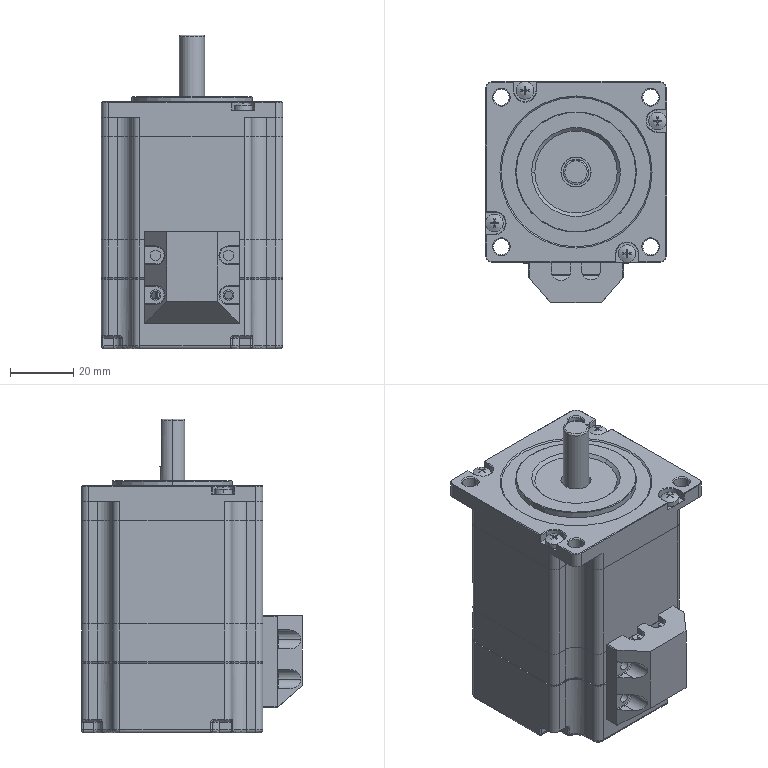Part | SolidWorks | 10 solids | 1966 faces | box 57.15 x 69.65 x 99 mm | volume 128417 mm3 | cone 1297 | cylinder 294 | plane 288 | spline 87 | commonest cylinder face diameters 1 x57 4.6 x40 0.6 x31 3.2 x27 9.5 x20 2 x16